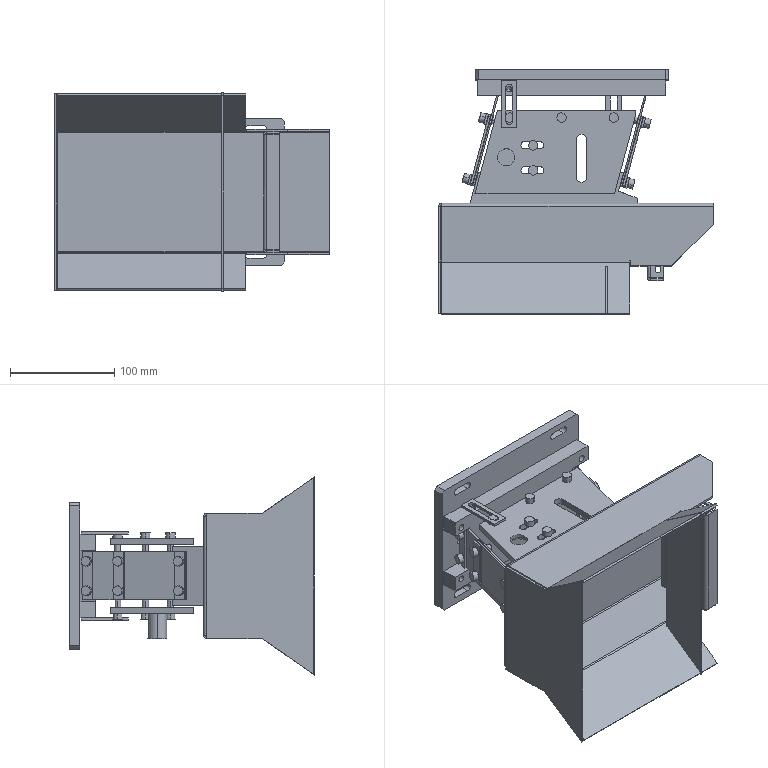Part | SolidWorks | 59 solids | 778 faces | box 263 x 234.482 x 189.769 mm | volume 1000691 mm3 | plane 376 | cylinder 368 | cone 30 | spline 4 | commonest cylinder face diameters 6.5 x128 6 x52 9 x44 5 x36 6.4 x26 4 x16